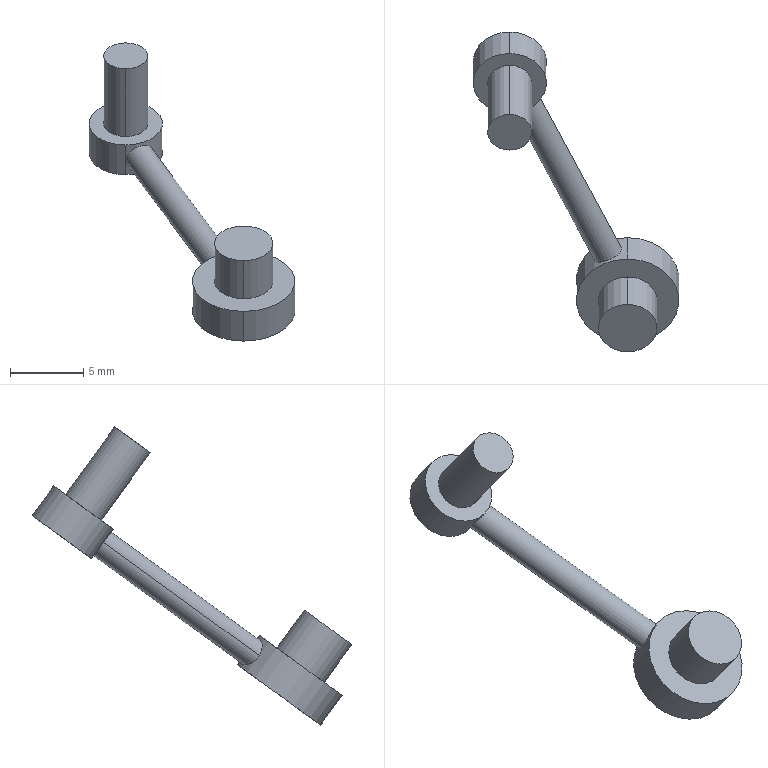Part | STEP file | Completa.sldasm-Part-144_Valor predeterminado | 1 solid | 22 faces | box 14.044 x 21.805 x 20.336 mm | volume 246.415 mm3 | cylinder 14 | plane 8 | commonest cylinder face diameters 3 x4 4 x4 2 x2 5 x2 7 x2